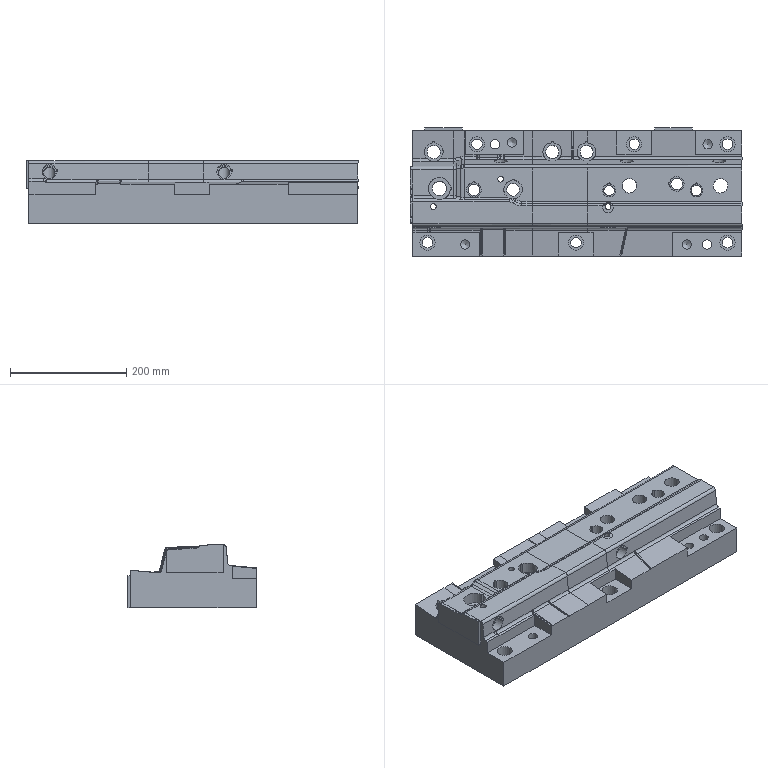Part | NX | features solid 2 | 1 solid | 284 faces | box 570.001 x 220 x 109.482 mm | volume 7618919 mm3 | cylinder 113 | plane 103 | spline 64 | cone 4 | commonest cylinder face diameters 10 x17 4 x14 12 x14 8 x10 18 x10 16 x7